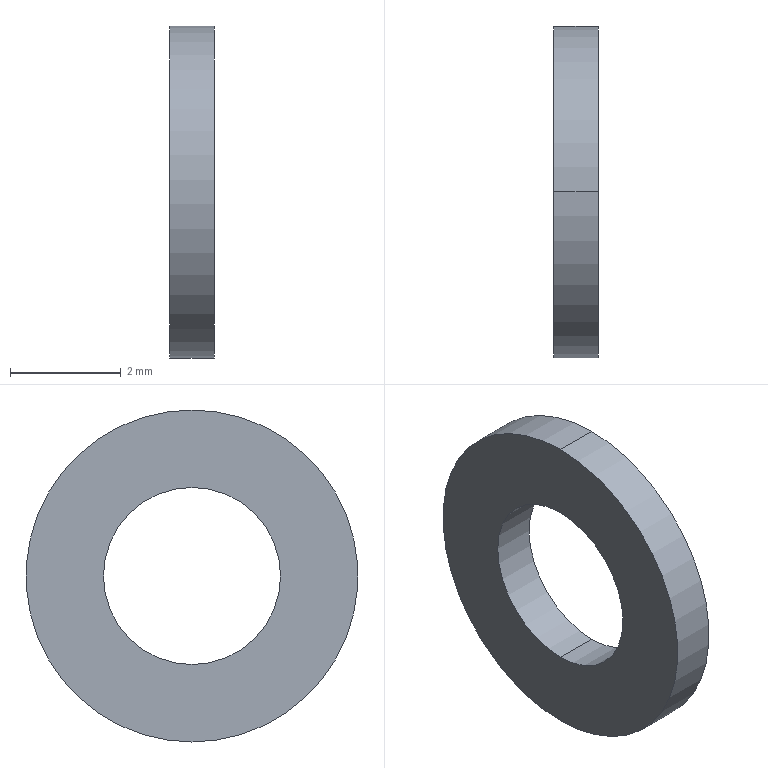Part | STEP file | 0230_313_PFW3 | 1 solid | 6 faces | box 0.8 x 6 x 6 mm | volume 16.185 mm3 | cylinder 4 | plane 2 | commonest cylinder face diameters 3.2 x2 6 x2
STEP:
#1=CARTESIAN_POINT('',(0.,0.,0.));
#2=DIRECTION('',(0.,0.,1.));
#3=DIRECTION('',(1.,0.,0.));
#4=AXIS2_PLACEMENT_3D('',#1,#2,#3);
#5=CARTESIAN_POINT('',(0.,0.,3.));
#6=VERTEX_POINT('',#5);
#7=CARTESIAN_POINT('',(0.,0.,-3.));
#8=VERTEX_POINT('',#7);
#9=CARTESIAN_POINT('',(0.,0.,0.));
#10=DIRECTION('',(-1.,0.,0.));
#11=DIRECTION('',(0.,0.,1.));
#12=AXIS2_PLACEMENT_3D('',#9,#10,#11);
#13=CIRCLE('',#12,3.);
#14=CARTESIAN_POINT('',(0.,0.,0.));
#15=DIRECTION('',(-1.,0.,0.));
#16=DIRECTION('',(0.,0.,1.));
#17=AXIS2_PLACEMENT_3D('',#14,#15,#16);
#18=CYLINDRICAL_SURFACE('',#17,3.);
#19=CARTESIAN_POINT('',(0.,0.));
#20=DIRECTION('',(1.,0.));
#21=VECTOR('',#20,1.);
#22=LINE('',#19,#21);
#23=(GEOMETRIC_REPRESENTATION_CONTEXT(2)PARAMETRIC_REPRESENTATION_CONTEXT()REPRESENTATION_CONTEXT('',''));
#24=DEFINITIONAL_REPRESENTATION('',(#22),#23);
#25=PCURVE('',#18,#24);
#26=CARTESIAN_POINT('',(0.,1.6,0.));
#27=DIRECTION('',(-1.,0.,0.));
#28=DIRECTION('',(0.,0.,1.));
#29=AXIS2_PLACEMENT_3D('',#26,#27,#28);
#30=PLANE('',#29);
#31=CARTESIAN_POINT('',(0.,-1.6));
#32=DIRECTION('',(1.,0.));
#33=AXIS2_PLACEMENT_2D('',#31,#32);
#34=CIRCLE('',#33,3.);
#35=(GEOMETRIC_REPRESENTATION_CONTEXT(2)PARAMETRIC_REPRESENTATION_CONTEXT()REPRESENTATION_CONTEXT('',''));
#36=DEFINITIONAL_REPRESENTATION('',(#34),#35);
#37=PCURVE('',#30,#36);
#38=SURFACE_CURVE('',#13,(#25,#37),.PCURVE_S1.);
#39=EDGE_CURVE('',#6,#8,#38,.T.);
#40=ORIENTED_EDGE('',*,*,#39,.T.);
#41=CARTESIAN_POINT('',(-0.8,0.,-3.));
#42=VERTEX_POINT('',#41);
#43=CARTESIAN_POINT('',(0.,0.,-3.));
#44=DIRECTION('',(-1.,0.,0.));
#45=VECTOR('',#44,1.);
#46=LINE('',#43,#45);
#47=CARTESIAN_POINT('',(3.142,0.));
#48=DIRECTION('',(0.,1.));
#49=VECTOR('',#48,1.);
#50=LINE('',#47,#49);
#51=(GEOMETRIC_REPRESENTATION_CONTEXT(2)PARAMETRIC_REPRESENTATION_CONTEXT()REPRESENTATION_CONTEXT('',''));
#52=DEFINITIONAL_REPRESENTATION('',(#50),#51);
#53=PCURVE('',#18,#52);
#54=CARTESIAN_POINT('',(0.,0.,0.));
#55=DIRECTION('',(-1.,0.,0.));
#56=DIRECTION('',(0.,0.,1.));
#57=AXIS2_PLACEMENT_3D('',#54,#55,#56);
#58=CYLINDRICAL_SURFACE('',#57,3.);
#59=CARTESIAN_POINT('',(3.142,0.));
#60=DIRECTION('',(0.,1.));
#61=VECTOR('',#60,1.);
#62=LINE('',#59,#61);
#63=(GEOMETRIC_REPRESENTATION_CONTEXT(2)PARAMETRIC_REPRESENTATION_CONTEXT()REPRESENTATION_CONTEXT('',''));
#64=DEFINITIONAL_REPRESENTATION('',(#62),#63);
#65=PCURVE('',#58,#64);
#66=SURFACE_CURVE('',#46,(#53,#65),.PCURVE_S1.);
#67=EDGE_CURVE('',#8,#42,#66,.T.);
#68=ORIENTED_EDGE('',*,*,#67,.T.);
#69=CARTESIAN_POINT('',(-0.8,0.,3.));
#70=VERTEX_POINT('',#69);
#71=CARTESIAN_POINT('',(-0.8,0.,0.));
#72=DIRECTION('',(1.,0.,0.));
#73=DIRECTION('',(0.,0.,1.));
#74=AXIS2_PLACEMENT_3D('',#71,#72,#73);
#75=CIRCLE('',#74,3.);
#76=CARTESIAN_POINT('',(6.283,0.8));
#77=DIRECTION('',(-1.,0.));
#78=VECTOR('',#77,1.);
#79=LINE('',#76,#78);
#80=(GEOMETRIC_REPRESENTATION_CONTEXT(2)PARAMETRIC_REPRESENTATION_CONTEXT()REPRESENTATION_CONTEXT('',''));
#81=DEFINITIONAL_REPRESENTATION('',(#79),#80);
#82=PCURVE('',#18,#81);
#83=CARTESIAN_POINT('',(-0.8,4.5,0.));
#84=DIRECTION('',(1.,0.,0.));
#85=DIRECTION('',(0.,0.,-1.));
#86=AXIS2_PLACEMENT_3D('',#83,#84,#85);
#87=PLANE('',#86);
#88=CARTESIAN_POINT('',(0.,-4.5));
#89=DIRECTION('',(-1.,0.));
#90=AXIS2_PLACEMENT_2D('',#88,#89);
#91=CIRCLE('',#90,3.);
#92=(GEOMETRIC_REPRESENTATION_CONTEXT(2)PARAMETRIC_REPRESENTATION_CONTEXT()REPRESENTATION_CONTEXT('',''));
#93=DEFINITIONAL_REPRESENTATION('',(#91),#92);
#94=PCURVE('',#87,#93);
#95=SURFACE_CURVE('',#75,(#82,#94),.PCURVE_S1.);
#96=EDGE_CURVE('',#42,#70,#95,.T.);
#97=ORIENTED_EDGE('',*,*,#96,.T.);
#98=CARTESIAN_POINT('',(0.,0.,3.));
#99=DIRECTION('',(-1.,0.,0.));
#100=VECTOR('',#99,1.);
#101=LINE('',#98,#100);
#102=CARTESIAN_POINT('',(0.,0.));
#103=DIRECTION('',(0.,1.));
#104=VECTOR('',#103,1.);
#105=LINE('',#102,#104);
#106=(GEOMETRIC_REPRESENTATION_CONTEXT(2)PARAMETRIC_REPRESENTATION_CONTEXT()REPRESENTATION_CONTEXT('',''));
#107=DEFINITIONAL_REPRESENTATION('',(#105),#106);
#108=PCURVE('',#18,#107);
#109=CARTESIAN_POINT('',(6.283,0.));
#110=DIRECTION('',(0.,1.));
#111=VECTOR('',#110,1.);
#112=LINE('',#109,#111);
#113=(GEOMETRIC_REPRESENTATION_CONTEXT(2)PARAMETRIC_REPRESENTATION_CONTEXT()REPRESENTATION_CONTEXT('',''));
#114=DEFINITIONAL_REPRESENTATION('',(#112),#113);
#115=PCURVE('',#58,#114);
#116=SURFACE_CURVE('',#101,(#108,#115),.PCURVE_S1.);
#117=EDGE_CURVE('',#6,#70,#116,.T.);
#118=ORIENTED_EDGE('',*,*,#117,.F.);
#119=EDGE_LOOP('',(#40,#68,#97,#118));
#120=FACE_BOUND('',#119,.T.);
#121=ADVANCED_FACE('',(#120),#18,.T.);
#122=CARTESIAN_POINT('',(0.,0.,1.6));
#123=VERTEX_POINT('',#122);
#124=CARTESIAN_POINT('',(-0.8,0.,1.6));
#125=VERTEX_POINT('',#124);
#126=CARTESIAN_POINT('',(-34.925,0.,1.6));
#127=DIRECTION('',(-1.,0.,0.));
#128=VECTOR('',#127,1.);
#129=LINE('',#126,#128);
#130=CARTESIAN_POINT('',(-34.925,0.,0.));
#131=DIRECTION('',(-1.,0.,0.));
#132=DIRECTION('',(0.,0.,1.));
#133=AXIS2_PLACEMENT_3D('',#130,#131,#132);
#134=CYLINDRICAL_SURFACE('',#133,1.6);
#135=CARTESIAN_POINT('',(6.283,0.));
#136=DIRECTION('',(0.,1.));
#137=VECTOR('',#136,1.);
#138=LINE('',#135,#137);
#139=(GEOMETRIC_REPRESENTATION_CONTEXT(2)PARAMETRIC_REPRESENTATION_CONTEXT()REPRESENTATION_CONTEXT('',''));
#140=DEFINITIONAL_REPRESENTATION('',(#138),#139);
#141=PCURVE('',#134,#140);
#142=CARTESIAN_POINT('',(-34.925,0.,0.));
#143=DIRECTION('',(-1.,0.,0.));
#144=DIRECTION('',(0.,0.,1.));
#145=AXIS2_PLACEMENT_3D('',#142,#143,#144);
#146=CYLINDRICAL_SURFACE('',#145,1.6);
#147=CARTESIAN_POINT('',(0.,0.));
#148=DIRECTION('',(0.,1.));
#149=VECTOR('',#148,1.);
#150=LINE('',#147,#149);
#151=(GEOMETRIC_REPRESENTATION_CONTEXT(2)PARAMETRIC_REPRESENTATION_CONTEXT()REPRESENTATION_CONTEXT('',''));
#152=DEFINITIONAL_REPRESENTATION('',(#150),#151);
#153=PCURVE('',#146,#152);
#154=SURFACE_CURVE('',#129,(#141,#153),.PCURVE_S1.);
#155=EDGE_CURVE('',#123,#125,#154,.T.);
#156=ORIENTED_EDGE('',*,*,#155,.T.);
#157=CARTESIAN_POINT('',(-0.8,0.,-1.6));
#158=VERTEX_POINT('',#157);
#159=CARTESIAN_POINT('',(-0.8,0.,0.));
#160=DIRECTION('',(-1.,0.,0.));
#161=DIRECTION('',(0.,0.,1.));
#162=AXIS2_PLACEMENT_3D('',#159,#160,#161);
#163=CIRCLE('',#162,1.6);
#164=CARTESIAN_POINT('',(0.,-34.125));
#165=DIRECTION('',(1.,0.));
#166=VECTOR('',#165,1.);
#167=LINE('',#164,#166);
#168=(GEOMETRIC_REPRESENTATION_CONTEXT(2)PARAMETRIC_REPRESENTATION_CONTEXT()REPRESENTATION_CONTEXT('',''));
#169=DEFINITIONAL_REPRESENTATION('',(#167),#168);
#170=PCURVE('',#134,#169);
#171=CARTESIAN_POINT('',(-1.6,-4.5));
#172=CARTESIAN_POINT('',(-1.6,-1.729));
#173=CARTESIAN_POINT('',(0.8,-3.114));
#174=CARTESIAN_POINT('',(3.2,-4.5));
#175=CARTESIAN_POINT('',(0.8,-5.886));
#176=CARTESIAN_POINT('',(-1.6,-7.271));
#177=CARTESIAN_POINT('',(-1.6,-4.5));
#178=(BOUNDED_CURVE()B_SPLINE_CURVE(2,(#171,#172,#173,#174,#175,#176,#177),.UNSPECIFIED.,.T.,.F.)B_SPLINE_CURVE_WITH_KNOTS((1,2,2,2,2,1),(-2.094,0.,2.094,4.189,6.283,8.378),.UNSPECIFIED.)CURVE()GEOMETRIC_REPRESENTATION_ITEM()RATIONAL_B_SPLINE_CURVE((1.,0.5,1.,0.5,1.,0.5,1.))REPRESENTATION_ITEM(''));
#179=(GEOMETRIC_REPRESENTATION_CONTEXT(2)PARAMETRIC_REPRESENTATION_CONTEXT()REPRESENTATION_CONTEXT('',''));
#180=DEFINITIONAL_REPRESENTATION('',(#178),#179);
#181=PCURVE('',#87,#180);
#182=SURFACE_CURVE('',#163,(#170,#181),.PCURVE_S1.);
#183=EDGE_CURVE('',#158,#125,#182,.T.);
#184=ORIENTED_EDGE('',*,*,#183,.F.);
#185=CARTESIAN_POINT('',(0.,0.,-1.6));
#186=VERTEX_POINT('',#185);
#187=CARTESIAN_POINT('',(-34.925,0.,-1.6));
#188=DIRECTION('',(-1.,0.,0.));
#189=VECTOR('',#188,1.);
#190=LINE('',#187,#189);
#191=CARTESIAN_POINT('',(3.142,0.));
#192=DIRECTION('',(0.,1.));
#193=VECTOR('',#192,1.);
#194=LINE('',#191,#193);
#195=(GEOMETRIC_REPRESENTATION_CONTEXT(2)PARAMETRIC_REPRESENTATION_CONTEXT()REPRESENTATION_CONTEXT('',''));
#196=DEFINITIONAL_REPRESENTATION('',(#194),#195);
#197=PCURVE('',#134,#196);
#198=CARTESIAN_POINT('',(3.142,0.));
#199=DIRECTION('',(0.,1.));
#200=VECTOR('',#199,1.);
#201=LINE('',#198,#200);
#202=(GEOMETRIC_REPRESENTATION_CONTEXT(2)PARAMETRIC_REPRESENTATION_CONTEXT()REPRESENTATION_CONTEXT('',''));
#203=DEFINITIONAL_REPRESENTATION('',(#201),#202);
#204=PCURVE('',#146,#203);
#205=SURFACE_CURVE('',#190,(#197,#204),.PCURVE_S1.);
#206=EDGE_CURVE('',#186,#158,#205,.T.);
#207=ORIENTED_EDGE('',*,*,#206,.F.);
#208=CARTESIAN_POINT('',(0.,0.,0.));
#209=DIRECTION('',(-1.,0.,0.));
#210=DIRECTION('',(0.,0.,1.));
#211=AXIS2_PLACEMENT_3D('',#208,#209,#210);
#212=CIRCLE('',#211,1.6);
#213=CARTESIAN_POINT('',(0.,-34.925));
#214=DIRECTION('',(1.,0.));
#215=VECTOR('',#214,1.);
#216=LINE('',#213,#215);
#217=(GEOMETRIC_REPRESENTATION_CONTEXT(2)PARAMETRIC_REPRESENTATION_CONTEXT()REPRESENTATION_CONTEXT('',''));
#218=DEFINITIONAL_REPRESENTATION('',(#216),#217);
#219=PCURVE('',#134,#218);
#220=CARTESIAN_POINT('',(0.,-1.6));
#221=DIRECTION('',(1.,0.));
#222=AXIS2_PLACEMENT_2D('',#220,#221);
#223=CIRCLE('',#222,1.6);
#224=(GEOMETRIC_REPRESENTATION_CONTEXT(2)PARAMETRIC_REPRESENTATION_CONTEXT()REPRESENTATION_CONTEXT('',''));
#225=DEFINITIONAL_REPRESENTATION('',(#223),#224);
#226=PCURVE('',#30,#225);
#227=SURFACE_CURVE('',#212,(#219,#226),.PCURVE_S1.);
#228=EDGE_CURVE('',#186,#123,#227,.T.);
#229=ORIENTED_EDGE('',*,*,#228,.T.);
#230=EDGE_LOOP('',(#156,#184,#207,#229));
#231=FACE_BOUND('',#230,.F.);
#232=ADVANCED_FACE('',(#231),#134,.F.);
#233=CARTESIAN_POINT('',(-0.8,0.,0.));
#234=DIRECTION('',(1.,0.,0.));
#235=DIRECTION('',(0.,0.,1.));
#236=AXIS2_PLACEMENT_3D('',#233,#234,#235);
#237=CIRCLE('',#236,3.);
#238=CARTESIAN_POINT('',(0.,-4.5));
#239=DIRECTION('',(-1.,0.));
#240=AXIS2_PLACEMENT_2D('',#238,#239);
#241=CIRCLE('',#240,3.);
#242=(GEOMETRIC_REPRESENTATION_CONTEXT(2)PARAMETRIC_REPRESENTATION_CONTEXT()REPRESENTATION_CONTEXT('',''));
#243=DEFINITIONAL_REPRESENTATION('',(#241),#242);
#244=PCURVE('',#87,#243);
#245=CARTESIAN_POINT('',(6.283,0.8));
#246=DIRECTION('',(-1.,0.));
#247=VECTOR('',#246,1.);
#248=LINE('',#245,#247);
#249=(GEOMETRIC_REPRESENTATION_CONTEXT(2)PARAMETRIC_REPRESENTATION_CONTEXT()REPRESENTATION_CONTEXT('',''));
#250=DEFINITIONAL_REPRESENTATION('',(#248),#249);
#251=PCURVE('',#58,#250);
#252=SURFACE_CURVE('',#237,(#244,#251),.PCURVE_S1.);
#253=EDGE_CURVE('',#70,#42,#252,.T.);
#254=ORIENTED_EDGE('',*,*,#253,.F.);
#255=ORIENTED_EDGE('',*,*,#96,.F.);
#256=EDGE_LOOP('',(#254,#255));
#257=FACE_BOUND('',#256,.T.);
#258=CARTESIAN_POINT('',(-0.8,0.,0.));
#259=DIRECTION('',(-1.,0.,0.));
#260=DIRECTION('',(0.,0.,1.));
#261=AXIS2_PLACEMENT_3D('',#258,#259,#260);
#262=CIRCLE('',#261,1.6);
#263=CARTESIAN_POINT('',(-1.6,-4.5));
#264=CARTESIAN_POINT('',(-1.6,-1.729));
#265=CARTESIAN_POINT('',(0.8,-3.114));
#266=CARTESIAN_POINT('',(3.2,-4.5));
#267=CARTESIAN_POINT('',(0.8,-5.886));
#268=CARTESIAN_POINT('',(-1.6,-7.271));
#269=CARTESIAN_POINT('',(-1.6,-4.5));
#270=(BOUNDED_CURVE()B_SPLINE_CURVE(2,(#263,#264,#265,#266,#267,#268,#269),.UNSPECIFIED.,.T.,.F.)B_SPLINE_CURVE_WITH_KNOTS((1,2,2,2,2,1),(-2.094,0.,2.094,4.189,6.283,8.378),.UNSPECIFIED.)CURVE()GEOMETRIC_REPRESENTATION_ITEM()RATIONAL_B_SPLINE_CURVE((1.,0.5,1.,0.5,1.,0.5,1.))REPRESENTATION_ITEM(''));
#271=(GEOMETRIC_REPRESENTATION_CONTEXT(2)PARAMETRIC_REPRESENTATION_CONTEXT()REPRESENTATION_CONTEXT('',''));
#272=DEFINITIONAL_REPRESENTATION('',(#270),#271);
#273=PCURVE('',#87,#272);
#274=CARTESIAN_POINT('',(0.,-34.125));
#275=DIRECTION('',(1.,0.));
#276=VECTOR('',#275,1.);
#277=LINE('',#274,#276);
#278=(GEOMETRIC_REPRESENTATION_CONTEXT(2)PARAMETRIC_REPRESENTATION_CONTEXT()REPRESENTATION_CONTEXT('',''));
#279=DEFINITIONAL_REPRESENTATION('',(#277),#278);
#280=PCURVE('',#146,#279);
#281=SURFACE_CURVE('',#262,(#273,#280),.PCURVE_S1.);
#282=EDGE_CURVE('',#125,#158,#281,.T.);
#283=ORIENTED_EDGE('',*,*,#282,.F.);
#284=ORIENTED_EDGE('',*,*,#183,.F.);
#285=EDGE_LOOP('',(#283,#284));
#286=FACE_BOUND('',#285,.T.);
#287=ADVANCED_FACE('',(#257,#286),#87,.F.);
#288=ORIENTED_EDGE('',*,*,#67,.F.);
#289=CARTESIAN_POINT('',(0.,0.,0.));
#290=DIRECTION('',(-1.,0.,0.));
#291=DIRECTION('',(0.,0.,1.));
#292=AXIS2_PLACEMENT_3D('',#289,#290,#291);
#293=CIRCLE('',#292,3.);
#294=CARTESIAN_POINT('',(0.,0.));
#295=DIRECTION('',(1.,0.));
#296=VECTOR('',#295,1.);
#297=LINE('',#294,#296);
#298=(GEOMETRIC_REPRESENTATION_CONTEXT(2)PARAMETRIC_REPRESENTATION_CONTEXT()REPRESENTATION_CONTEXT('',''));
#299=DEFINITIONAL_REPRESENTATION('',(#297),#298);
#300=PCURVE('',#58,#299);
#301=CARTESIAN_POINT('',(0.,-1.6));
#302=DIRECTION('',(1.,0.));
#303=AXIS2_PLACEMENT_2D('',#301,#302);
#304=CIRCLE('',#303,3.);
#305=(GEOMETRIC_REPRESENTATION_CONTEXT(2)PARAMETRIC_REPRESENTATION_CONTEXT()REPRESENTATION_CONTEXT('',''));
#306=DEFINITIONAL_REPRESENTATION('',(#304),#305);
#307=PCURVE('',#30,#306);
#308=SURFACE_CURVE('',#293,(#300,#307),.PCURVE_S1.);
#309=EDGE_CURVE('',#8,#6,#308,.T.);
#310=ORIENTED_EDGE('',*,*,#309,.T.);
#311=ORIENTED_EDGE('',*,*,#117,.T.);
#312=ORIENTED_EDGE('',*,*,#253,.T.);
#313=EDGE_LOOP('',(#288,#310,#311,#312));
#314=FACE_BOUND('',#313,.T.);
#315=ADVANCED_FACE('',(#314),#58,.T.);
#316=ORIENTED_EDGE('',*,*,#282,.F.);
#317=ORIENTED_EDGE('',*,*,#155,.F.);
#318=CARTESIAN_POINT('',(0.,0.,0.));
#319=DIRECTION('',(-1.,0.,0.));
#320=DIRECTION('',(0.,0.,1.));
#321=AXIS2_PLACEMENT_3D('',#318,#319,#320);
#322=CIRCLE('',#321,1.6);
#323=CARTESIAN_POINT('',(0.,-34.925));
#324=DIRECTION('',(1.,0.));
#325=VECTOR('',#324,1.);
#326=LINE('',#323,#325);
#327=(GEOMETRIC_REPRESENTATION_CONTEXT(2)PARAMETRIC_REPRESENTATION_CONTEXT()REPRESENTATION_CONTEXT('',''));
#328=DEFINITIONAL_REPRESENTATION('',(#326),#327);
#329=PCURVE('',#146,#328);
#330=CARTESIAN_POINT('',(0.,-1.6));
#331=DIRECTION('',(1.,0.));
#332=AXIS2_PLACEMENT_2D('',#330,#331);
#333=CIRCLE('',#332,1.6);
#334=(GEOMETRIC_REPRESENTATION_CONTEXT(2)PARAMETRIC_REPRESENTATION_CONTEXT()REPRESENTATION_CONTEXT('',''));
#335=DEFINITIONAL_REPRESENTATION('',(#333),#334);
#336=PCURVE('',#30,#335);
#337=SURFACE_CURVE('',#322,(#329,#336),.PCURVE_S1.);
#338=EDGE_CURVE('',#123,#186,#337,.T.);
#339=ORIENTED_EDGE('',*,*,#338,.T.);
#340=ORIENTED_EDGE('',*,*,#206,.T.);
#341=EDGE_LOOP('',(#316,#317,#339,#340));
#342=FACE_BOUND('',#341,.F.);
#343=ADVANCED_FACE('',(#342),#146,.F.);
#344=ORIENTED_EDGE('',*,*,#39,.F.);
#345=ORIENTED_EDGE('',*,*,#309,.F.);
#346=EDGE_LOOP('',(#344,#345));
#347=FACE_BOUND('',#346,.T.);
#348=ORIENTED_EDGE('',*,*,#338,.T.);
#349=ORIENTED_EDGE('',*,*,#228,.T.);
#350=EDGE_LOOP('',(#348,#349));
#351=FACE_BOUND('',#350,.T.);
#352=ADVANCED_FACE('',(#347,#351),#30,.F.);
#353=CLOSED_SHELL('',(#121,#232,#287,#315,#343,#352));
#354=MANIFOLD_SOLID_BREP('',#353);
#355=(LENGTH_UNIT()NAMED_UNIT(*)SI_UNIT(.MILLI.,.METRE.));
#356=UNCERTAINTY_MEASURE_WITH_UNIT(LENGTH_MEASURE(0.0000001),#355,'','');
#357=(NAMED_UNIT(*)PLANE_ANGLE_UNIT()SI_UNIT($,.RADIAN.));
#358=(NAMED_UNIT(*)SI_UNIT($,.STERADIAN.)SOLID_ANGLE_UNIT());
#359=(GEOMETRIC_REPRESENTATION_CONTEXT(3)GLOBAL_UNCERTAINTY_ASSIGNED_CONTEXT((#356))GLOBAL_UNIT_ASSIGNED_CONTEXT((#355,#357,#358))REPRESENTATION_CONTEXT('',''));
#360=ADVANCED_BREP_SHAPE_REPRESENTATION('',(#4,#354),#359);